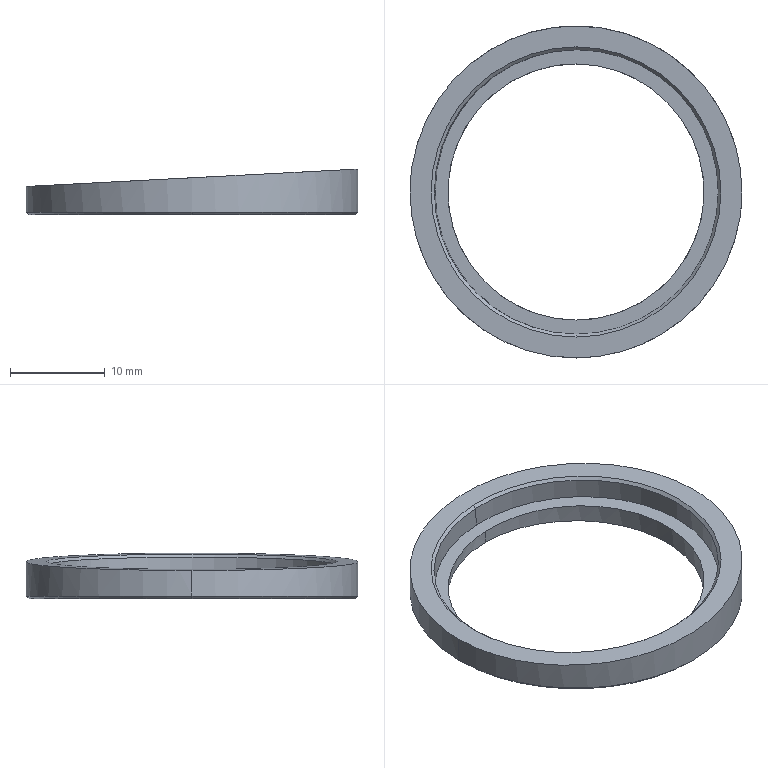Part | STEP file | TCHK-2D-D30-BB-4.stp.STEP | 1 solid | 14 faces | box 35 x 35 x 4.834 mm | volume 1185 mm3 | cylinder 6 | cone 5 | plane 3 | commonest cylinder face diameters 27 x2 30 x2 35 x2
STEP:
#1=CARTESIAN_POINT('',(0.,13.5,0.));
#2=VERTEX_POINT('',#1);
#3=CARTESIAN_POINT('',(0.,-13.5,0.));
#4=VERTEX_POINT('',#3);
#5=CARTESIAN_POINT('',(0.,0.,0.));
#6=DIRECTION('',(0.,0.,-1.));
#7=DIRECTION('',(0.,1.,0.));
#8=AXIS2_PLACEMENT_3D('',#5,#6,#7);
#9=CIRCLE('',#8,13.5);
#10=EDGE_CURVE('',#2,#4,#9,.T.);
#11=ORIENTED_EDGE('',*,*,#10,.F.);
#12=CARTESIAN_POINT('',(0.,0.,0.));
#13=DIRECTION('',(0.,0.,-1.));
#14=DIRECTION('',(0.,-1.,0.));
#15=AXIS2_PLACEMENT_3D('',#12,#13,#14);
#16=CIRCLE('',#15,13.5);
#17=EDGE_CURVE('',#4,#2,#16,.T.);
#18=ORIENTED_EDGE('',*,*,#17,.F.);
#19=EDGE_LOOP('',(#11,#18));
#20=FACE_BOUND('',#19,.T.);
#21=CARTESIAN_POINT('',(17.2,0.,0.000000446));
#22=VERTEX_POINT('',#21);
#23=CARTESIAN_POINT('',(0.,-17.2,0.000000446));
#24=VERTEX_POINT('',#23);
#25=CARTESIAN_POINT('',(0.,0.,0.000000446));
#26=DIRECTION('',(0.,0.,-1.));
#27=DIRECTION('',(1.,0.,0.));
#28=AXIS2_PLACEMENT_3D('',#25,#26,#27);
#29=CIRCLE('',#28,17.2);
#30=EDGE_CURVE('',#22,#24,#29,.T.);
#31=ORIENTED_EDGE('',*,*,#30,.T.);
#32=CARTESIAN_POINT('',(-17.2,0.,0.000000446));
#33=VERTEX_POINT('',#32);
#34=CARTESIAN_POINT('',(0.,0.,0.000000446));
#35=DIRECTION('',(0.,0.,-1.));
#36=DIRECTION('',(1.,0.,0.));
#37=AXIS2_PLACEMENT_3D('',#34,#35,#36);
#38=CIRCLE('',#37,17.2);
#39=EDGE_CURVE('',#24,#33,#38,.T.);
#40=ORIENTED_EDGE('',*,*,#39,.T.);
#41=CARTESIAN_POINT('',(0.,0.,0.000000446));
#42=DIRECTION('',(0.,0.,-1.));
#43=DIRECTION('',(-1.,0.,0.));
#44=AXIS2_PLACEMENT_3D('',#41,#42,#43);
#45=CIRCLE('',#44,17.2);
#46=EDGE_CURVE('',#33,#22,#45,.T.);
#47=ORIENTED_EDGE('',*,*,#46,.T.);
#48=EDGE_LOOP('',(#31,#40,#47));
#49=FACE_OUTER_BOUND('',#48,.T.);
#50=CARTESIAN_POINT('',(0.,0.,0.));
#51=DIRECTION('',(0.,0.,1.));
#52=DIRECTION('',(1.,0.,0.));
#53=AXIS2_PLACEMENT_3D('',#50,#51,#52);
#54=PLANE('',#53);
#55=ADVANCED_FACE('',(#20,#49),#54,.F.);
#56=CARTESIAN_POINT('',(-17.5,0.,0.3));
#57=VERTEX_POINT('',#56);
#58=CARTESIAN_POINT('',(-17.2,-0.000000003,0.000000796));
#59=DIRECTION('',(-0.7071,0.000000001,0.7071));
#60=VECTOR('',#59,1000.);
#61=LINE('',#58,#60);
#62=EDGE_CURVE('',#33,#57,#61,.T.);
#63=ORIENTED_EDGE('',*,*,#62,.T.);
#64=CARTESIAN_POINT('',(17.5,0.,0.3));
#65=VERTEX_POINT('',#64);
#66=CARTESIAN_POINT('',(0.,0.,0.3));
#67=DIRECTION('',(0.,0.,-1.));
#68=DIRECTION('',(-1.,0.,0.));
#69=AXIS2_PLACEMENT_3D('',#66,#67,#68);
#70=CIRCLE('',#69,17.5);
#71=EDGE_CURVE('',#57,#65,#70,.T.);
#72=ORIENTED_EDGE('',*,*,#71,.T.);
#73=CARTESIAN_POINT('',(17.2,0.000000003,0.000000796));
#74=DIRECTION('',(0.7071,-0.000000001,0.7071));
#75=VECTOR('',#74,1000.);
#76=LINE('',#73,#75);
#77=EDGE_CURVE('',#22,#65,#76,.T.);
#78=ORIENTED_EDGE('',*,*,#77,.F.);
#79=ORIENTED_EDGE('',*,*,#46,.F.);
#80=EDGE_LOOP('',(#63,#72,#78,#79));
#81=FACE_OUTER_BOUND('',#80,.T.);
#82=CARTESIAN_POINT('',(0.,0.,0.15));
#83=DIRECTION('',(0.,0.,1.));
#84=DIRECTION('',(0.,-1.,0.));
#85=AXIS2_PLACEMENT_3D('',#82,#83,#84);
#86=CONICAL_SURFACE('',#85,17.35,0.7854);
#87=ADVANCED_FACE('',(#81),#86,.T.);
#88=CARTESIAN_POINT('',(0.,-17.5,0.3));
#89=VERTEX_POINT('',#88);
#90=CARTESIAN_POINT('',(0.,-17.35,0.15));
#91=DIRECTION('',(0.,-0.7071,0.7071));
#92=VECTOR('',#91,1000.);
#93=LINE('',#90,#92);
#94=EDGE_CURVE('',#24,#89,#93,.T.);
#95=ORIENTED_EDGE('',*,*,#94,.F.);
#96=ORIENTED_EDGE('',*,*,#30,.F.);
#97=ORIENTED_EDGE('',*,*,#77,.T.);
#98=CARTESIAN_POINT('',(0.,0.,0.3));
#99=DIRECTION('',(0.,0.,-1.));
#100=DIRECTION('',(1.,0.,0.));
#101=AXIS2_PLACEMENT_3D('',#98,#99,#100);
#102=CIRCLE('',#101,17.5);
#103=EDGE_CURVE('',#65,#89,#102,.T.);
#104=ORIENTED_EDGE('',*,*,#103,.T.);
#105=EDGE_LOOP('',(#95,#96,#97,#104));
#106=FACE_OUTER_BOUND('',#105,.T.);
#107=CARTESIAN_POINT('',(0.,0.,0.15));
#108=DIRECTION('',(0.,0.,1.));
#109=DIRECTION('',(0.,-1.,0.));
#110=AXIS2_PLACEMENT_3D('',#107,#108,#109);
#111=CONICAL_SURFACE('',#110,17.35,0.7854);
#112=ADVANCED_FACE('',(#106),#111,.T.);
#113=CARTESIAN_POINT('',(17.5,0.,4.834));
#114=VERTEX_POINT('',#113);
#115=CARTESIAN_POINT('',(17.5,0.000000002,0.3));
#116=DIRECTION('',(0.000000134,0.,1.));
#117=VECTOR('',#116,1000.);
#118=LINE('',#115,#117);
#119=EDGE_CURVE('',#65,#114,#118,.T.);
#120=ORIENTED_EDGE('',*,*,#119,.T.);
#121=CARTESIAN_POINT('',(-17.5,0.,3.));
#122=VERTEX_POINT('',#121);
#123=CARTESIAN_POINT('',(-17.5,0.,3.));
#124=CARTESIAN_POINT('',(-17.5,-0.5353,3.));
#125=CARTESIAN_POINT('',(-17.463,-1.335,3.002));
#126=CARTESIAN_POINT('',(-17.357,-2.262,3.007));
#127=CARTESIAN_POINT('',(-17.288,-2.723,3.011));
#128=CARTESIAN_POINT('',(-17.249,-2.954,3.013));
#129=CARTESIAN_POINT('',(-17.232,-3.053,3.014));
#130=CARTESIAN_POINT('',(-17.22,-3.119,3.015));
#131=CARTESIAN_POINT('',(-17.214,-3.149,3.015));
#132=CARTESIAN_POINT('',(-17.105,-3.742,3.021));
#133=CARTESIAN_POINT('',(-16.91,-4.568,3.031));
#134=CARTESIAN_POINT('',(-16.614,-5.512,3.046));
#135=CARTESIAN_POINT('',(-16.448,-5.978,3.055));
#136=CARTESIAN_POINT('',(-16.361,-6.21,3.06));
#137=CARTESIAN_POINT('',(-16.323,-6.31,3.062));
#138=CARTESIAN_POINT('',(-16.297,-6.376,3.063));
#139=CARTESIAN_POINT('',(-16.285,-6.407,3.064));
#140=CARTESIAN_POINT('',(-16.054,-6.991,3.076));
#141=CARTESIAN_POINT('',(-15.687,-7.796,3.095));
#142=CARTESIAN_POINT('',(-15.191,-8.698,3.121));
#143=CARTESIAN_POINT('',(-14.925,-9.14,3.135));
#144=CARTESIAN_POINT('',(-14.807,-9.328,3.141));
#145=CARTESIAN_POINT('',(-14.728,-9.452,3.145));
#146=CARTESIAN_POINT('',(-14.689,-9.513,3.147));
#147=CARTESIAN_POINT('',(-13.987,-10.587,3.184));
#148=CARTESIAN_POINT('',(-13.228,-11.521,3.224));
#149=CARTESIAN_POINT('',(-11.948,-12.801,3.291));
#150=CARTESIAN_POINT('',(-11.278,-13.406,3.326));
#151=CARTESIAN_POINT('',(-10.444,-14.047,3.37));
#152=CARTESIAN_POINT('',(-10.015,-14.353,3.392));
#153=CARTESIAN_POINT('',(-9.828,-14.48,3.402));
#154=CARTESIAN_POINT('',(-9.702,-14.564,3.409));
#155=CARTESIAN_POINT('',(-9.638,-14.607,3.412));
#156=CARTESIAN_POINT('',(-9.082,-14.971,3.441));
#157=CARTESIAN_POINT('',(-8.319,-15.416,3.481));
#158=CARTESIAN_POINT('',(-7.393,-15.867,3.53));
#159=CARTESIAN_POINT('',(-6.92,-16.075,3.554));
#160=CARTESIAN_POINT('',(-6.682,-16.174,3.567));
#161=CARTESIAN_POINT('',(-6.579,-16.216,3.572));
#162=CARTESIAN_POINT('',(-6.51,-16.244,3.576));
#163=CARTESIAN_POINT('',(-6.475,-16.258,3.578));
#164=CARTESIAN_POINT('',(-5.915,-16.48,3.607));
#165=CARTESIAN_POINT('',(-5.113,-16.754,3.649));
#166=CARTESIAN_POINT('',(-4.155,-17.004,3.699));
#167=CARTESIAN_POINT('',(-3.672,-17.112,3.725));
#168=CARTESIAN_POINT('',(-3.428,-17.161,3.737));
#169=CARTESIAN_POINT('',(-3.324,-17.181,3.743));
#170=CARTESIAN_POINT('',(-3.254,-17.195,3.747));
#171=CARTESIAN_POINT('',(-3.217,-17.202,3.749));
#172=CARTESIAN_POINT('',(-2.133,-17.403,3.805));
#173=CARTESIAN_POINT('',(-1.07,-17.5,3.861));
#174=CARTESIAN_POINT('',(0.535,-17.5,3.945));
#175=CARTESIAN_POINT('',(1.334,-17.464,3.987));
#176=CARTESIAN_POINT('',(2.261,-17.357,4.036));
#177=CARTESIAN_POINT('',(2.723,-17.288,4.06));
#178=CARTESIAN_POINT('',(2.954,-17.249,4.072));
#179=CARTESIAN_POINT('',(3.053,-17.232,4.077));
#180=CARTESIAN_POINT('',(3.119,-17.22,4.081));
#181=CARTESIAN_POINT('',(3.149,-17.214,4.082));
#182=CARTESIAN_POINT('',(3.743,-17.105,4.113));
#183=CARTESIAN_POINT('',(4.569,-16.91,4.157));
#184=CARTESIAN_POINT('',(5.512,-16.614,4.206));
#185=CARTESIAN_POINT('',(5.978,-16.448,4.23));
#186=CARTESIAN_POINT('',(6.21,-16.361,4.243));
#187=CARTESIAN_POINT('',(6.31,-16.323,4.248));
#188=CARTESIAN_POINT('',(6.376,-16.297,4.251));
#189=CARTESIAN_POINT('',(6.407,-16.285,4.253));
#190=CARTESIAN_POINT('',(6.992,-16.054,4.284));
#191=CARTESIAN_POINT('',(7.796,-15.687,4.326));
#192=CARTESIAN_POINT('',(8.698,-15.19,4.373));
#193=CARTESIAN_POINT('',(9.14,-14.925,4.396));
#194=CARTESIAN_POINT('',(9.328,-14.807,4.406));
#195=CARTESIAN_POINT('',(9.452,-14.728,4.413));
#196=CARTESIAN_POINT('',(9.513,-14.689,4.416));
#197=CARTESIAN_POINT('',(10.587,-13.987,4.472));
#198=CARTESIAN_POINT('',(11.521,-13.228,4.521));
#199=CARTESIAN_POINT('',(12.801,-11.948,4.588));
#200=CARTESIAN_POINT('',(13.405,-11.278,4.62));
#201=CARTESIAN_POINT('',(14.047,-10.444,4.653));
#202=CARTESIAN_POINT('',(14.353,-10.015,4.669));
#203=CARTESIAN_POINT('',(14.48,-9.828,4.676));
#204=CARTESIAN_POINT('',(14.564,-9.702,4.68));
#205=CARTESIAN_POINT('',(14.607,-9.638,4.683));
#206=CARTESIAN_POINT('',(14.971,-9.082,4.702));
#207=CARTESIAN_POINT('',(15.416,-8.319,4.725));
#208=CARTESIAN_POINT('',(15.867,-7.393,4.749));
#209=CARTESIAN_POINT('',(16.075,-6.92,4.76));
#210=CARTESIAN_POINT('',(16.174,-6.682,4.765));
#211=CARTESIAN_POINT('',(16.216,-6.579,4.767));
#212=CARTESIAN_POINT('',(16.244,-6.51,4.768));
#213=CARTESIAN_POINT('',(16.258,-6.475,4.769));
#214=CARTESIAN_POINT('',(16.48,-5.915,4.781));
#215=CARTESIAN_POINT('',(16.754,-5.112,4.795));
#216=CARTESIAN_POINT('',(17.004,-4.155,4.808));
#217=CARTESIAN_POINT('',(17.112,-3.672,4.814));
#218=CARTESIAN_POINT('',(17.161,-3.428,4.817));
#219=CARTESIAN_POINT('',(17.181,-3.324,4.818));
#220=CARTESIAN_POINT('',(17.195,-3.254,4.818));
#221=CARTESIAN_POINT('',(17.202,-3.217,4.819));
#222=CARTESIAN_POINT('',(17.403,-2.133,4.829));
#223=CARTESIAN_POINT('',(17.5,-1.071,4.834));
#224=CARTESIAN_POINT('',(17.5,0.,4.834));
#225=B_SPLINE_CURVE_WITH_KNOTS('',3,(#123,#124,#125,#126,#127,#128,#129,#130,#131,#132,#133,#134,#135,#136,#137,#138,#139,#140,#141,#142,#143,#144,#145,#146,#147,#148,#149,#150,#151,#152,#153,#154,#155,#156,#157,#158,#159,#160,#161,#162,#163,#164,#165,#166,#167,#168,#169,#170,#171,#172,#173,#174,#175,#176,#177,#178,#179,#180,#181,#182,#183,#184,#185,#186,#187,#188,#189,#190,#191,#192,#193,#194,#195,#196,#197,#198,#199,#200,#201,#202,#203,#204,#205,#206,#207,#208,#209,#210,#211,#212,#213,#214,#215,#216,#217,#218,#219,#220,#221,#222,#223,#224),.UNSPECIFIED.,.F.,.F.,(4,1,1,1,1,2,2,1,1,1,1,2,2,1,1,1,2,2,2,1,1,1,2,2,1,1,1,1,2,2,1,1,1,1,2,2,2,1,1,1,1,2,2,1,1,1,1,2,2,1,1,1,2,2,2,1,1,1,2,2,1,1,1,1,2,2,1,1,1,1,2,2,4),(0.,0.03125,0.04687,0.05469,0.05859,0.06055,0.0625,0.09375,0.1094,0.1172,0.1211,0.123,0.125,0.1562,0.1719,0.1797,0.1836,0.1875,0.25,0.2812,0.2969,0.3047,0.3086,0.3125,0.3437,0.3594,0.3672,0.3711,0.373,0.375,0.4062,0.4219,0.4297,0.4336,0.4355,0.4375,0.5,0.5312,0.5469,0.5547,0.5586,0.5605,0.5625,0.5937,0.6094,0.6172,0.6211,0.623,0.625,0.6562,0.6719,0.6797,0.6836,0.6875,0.75,0.7812,0.7969,0.8047,0.8086,0.8125,0.8437,0.8594,0.8672,0.8711,0.873,0.875,0.9062,0.9219,0.9297,0.9336,0.9355,0.9375,1.),.UNSPECIFIED.);
#226=EDGE_CURVE('',#122,#114,#225,.T.);
#227=ORIENTED_EDGE('',*,*,#226,.F.);
#228=CARTESIAN_POINT('',(-17.5,-0.000000002,0.3));
#229=DIRECTION('',(-0.000000225,0.000000001,1.));
#230=VECTOR('',#229,1000.);
#231=LINE('',#228,#230);
#232=EDGE_CURVE('',#57,#122,#231,.T.);
#233=ORIENTED_EDGE('',*,*,#232,.F.);
#234=CARTESIAN_POINT('',(0.,0.,0.3));
#235=DIRECTION('',(0.,0.,-1.));
#236=DIRECTION('',(1.,0.,0.));
#237=AXIS2_PLACEMENT_3D('',#234,#235,#236);
#238=CIRCLE('',#237,17.5);
#239=EDGE_CURVE('',#89,#57,#238,.T.);
#240=ORIENTED_EDGE('',*,*,#239,.F.);
#241=ORIENTED_EDGE('',*,*,#103,.F.);
#242=EDGE_LOOP('',(#120,#227,#233,#240,#241));
#243=FACE_OUTER_BOUND('',#242,.T.);
#244=CARTESIAN_POINT('',(0.,0.,0.));
#245=DIRECTION('',(0.,0.,1.));
#246=DIRECTION('',(1.,0.,0.));
#247=AXIS2_PLACEMENT_3D('',#244,#245,#246);
#248=CYLINDRICAL_SURFACE('',#247,17.5);
#249=ADVANCED_FACE('',(#243),#248,.T.);
#250=ORIENTED_EDGE('',*,*,#232,.T.);
#251=CARTESIAN_POINT('',(17.5,0.,4.834));
#252=CARTESIAN_POINT('',(17.5,0.5353,4.834));
#253=CARTESIAN_POINT('',(17.463,1.335,4.832));
#254=CARTESIAN_POINT('',(17.357,2.262,4.827));
#255=CARTESIAN_POINT('',(17.288,2.723,4.823));
#256=CARTESIAN_POINT('',(17.249,2.954,4.821));
#257=CARTESIAN_POINT('',(17.232,3.053,4.82));
#258=CARTESIAN_POINT('',(17.22,3.119,4.82));
#259=CARTESIAN_POINT('',(17.214,3.149,4.819));
#260=CARTESIAN_POINT('',(17.105,3.742,4.814));
#261=CARTESIAN_POINT('',(16.91,4.568,4.803));
#262=CARTESIAN_POINT('',(16.614,5.512,4.788));
#263=CARTESIAN_POINT('',(16.448,5.978,4.779));
#264=CARTESIAN_POINT('',(16.361,6.21,4.775));
#265=CARTESIAN_POINT('',(16.323,6.31,4.773));
#266=CARTESIAN_POINT('',(16.297,6.376,4.771));
#267=CARTESIAN_POINT('',(16.285,6.407,4.771));
#268=CARTESIAN_POINT('',(16.054,6.991,4.758));
#269=CARTESIAN_POINT('',(15.687,7.796,4.739));
#270=CARTESIAN_POINT('',(15.191,8.698,4.713));
#271=CARTESIAN_POINT('',(14.925,9.14,4.699));
#272=CARTESIAN_POINT('',(14.807,9.328,4.693));
#273=CARTESIAN_POINT('',(14.728,9.452,4.689));
#274=CARTESIAN_POINT('',(14.689,9.513,4.687));
#275=CARTESIAN_POINT('',(13.987,10.587,4.65));
#276=CARTESIAN_POINT('',(13.228,11.521,4.61));
#277=CARTESIAN_POINT('',(11.948,12.801,4.543));
#278=CARTESIAN_POINT('',(11.278,13.406,4.508));
#279=CARTESIAN_POINT('',(10.444,14.047,4.464));
#280=CARTESIAN_POINT('',(10.015,14.353,4.442));
#281=CARTESIAN_POINT('',(9.828,14.48,4.432));
#282=CARTESIAN_POINT('',(9.702,14.564,4.426));
#283=CARTESIAN_POINT('',(9.638,14.607,4.422));
#284=CARTESIAN_POINT('',(9.082,14.971,4.393));
#285=CARTESIAN_POINT('',(8.319,15.416,4.353));
#286=CARTESIAN_POINT('',(7.393,15.867,4.305));
#287=CARTESIAN_POINT('',(6.92,16.075,4.28));
#288=CARTESIAN_POINT('',(6.682,16.174,4.267));
#289=CARTESIAN_POINT('',(6.579,16.216,4.262));
#290=CARTESIAN_POINT('',(6.51,16.244,4.258));
#291=CARTESIAN_POINT('',(6.475,16.258,4.256));
#292=CARTESIAN_POINT('',(5.915,16.48,4.227));
#293=CARTESIAN_POINT('',(5.113,16.754,4.185));
#294=CARTESIAN_POINT('',(4.155,17.004,4.135));
#295=CARTESIAN_POINT('',(3.672,17.112,4.11));
#296=CARTESIAN_POINT('',(3.428,17.161,4.097));
#297=CARTESIAN_POINT('',(3.324,17.181,4.091));
#298=CARTESIAN_POINT('',(3.254,17.195,4.088));
#299=CARTESIAN_POINT('',(3.217,17.202,4.086));
#300=CARTESIAN_POINT('',(2.133,17.403,4.029));
#301=CARTESIAN_POINT('',(1.07,17.5,3.973));
#302=CARTESIAN_POINT('',(-0.535,17.5,3.889));
#303=CARTESIAN_POINT('',(-1.334,17.464,3.847));
#304=CARTESIAN_POINT('',(-2.261,17.357,3.799));
#305=CARTESIAN_POINT('',(-2.723,17.288,3.774));
#306=CARTESIAN_POINT('',(-2.954,17.249,3.762));
#307=CARTESIAN_POINT('',(-3.053,17.232,3.757));
#308=CARTESIAN_POINT('',(-3.119,17.22,3.754));
#309=CARTESIAN_POINT('',(-3.149,17.214,3.752));
#310=CARTESIAN_POINT('',(-3.743,17.105,3.721));
#311=CARTESIAN_POINT('',(-4.569,16.91,3.678));
#312=CARTESIAN_POINT('',(-5.512,16.614,3.628));
#313=CARTESIAN_POINT('',(-5.978,16.448,3.604));
#314=CARTESIAN_POINT('',(-6.21,16.361,3.592));
#315=CARTESIAN_POINT('',(-6.31,16.323,3.586));
#316=CARTESIAN_POINT('',(-6.376,16.297,3.583));
#317=CARTESIAN_POINT('',(-6.407,16.285,3.581));
#318=CARTESIAN_POINT('',(-6.992,16.054,3.551));
#319=CARTESIAN_POINT('',(-7.796,15.687,3.509));
#320=CARTESIAN_POINT('',(-8.698,15.19,3.461));
#321=CARTESIAN_POINT('',(-9.14,14.925,3.438));
#322=CARTESIAN_POINT('',(-9.328,14.807,3.428));
#323=CARTESIAN_POINT('',(-9.452,14.728,3.422));
#324=CARTESIAN_POINT('',(-9.513,14.689,3.419));
#325=CARTESIAN_POINT('',(-10.587,13.987,3.362));
#326=CARTESIAN_POINT('',(-11.521,13.228,3.313));
#327=CARTESIAN_POINT('',(-12.801,11.948,3.246));
#328=CARTESIAN_POINT('',(-13.405,11.278,3.215));
#329=CARTESIAN_POINT('',(-14.047,10.444,3.181));
#330=CARTESIAN_POINT('',(-14.353,10.015,3.165));
#331=CARTESIAN_POINT('',(-14.48,9.828,3.158));
#332=CARTESIAN_POINT('',(-14.564,9.702,3.154));
#333=CARTESIAN_POINT('',(-14.607,9.638,3.152));
#334=CARTESIAN_POINT('',(-14.971,9.082,3.133));
#335=CARTESIAN_POINT('',(-15.416,8.319,3.109));
#336=CARTESIAN_POINT('',(-15.867,7.393,3.086));
#337=CARTESIAN_POINT('',(-16.075,6.92,3.075));
#338=CARTESIAN_POINT('',(-16.174,6.682,3.069));
#339=CARTESIAN_POINT('',(-16.216,6.579,3.067));
#340=CARTESIAN_POINT('',(-16.244,6.51,3.066));
#341=CARTESIAN_POINT('',(-16.258,6.475,3.065));
#342=CARTESIAN_POINT('',(-16.48,5.915,3.053));
#343=CARTESIAN_POINT('',(-16.754,5.112,3.039));
#344=CARTESIAN_POINT('',(-17.004,4.155,3.026));
#345=CARTESIAN_POINT('',(-17.112,3.672,3.02));
#346=CARTESIAN_POINT('',(-17.161,3.428,3.018));
#347=CARTESIAN_POINT('',(-17.181,3.324,3.017));
#348=CARTESIAN_POINT('',(-17.195,3.254,3.016));
#349=CARTESIAN_POINT('',(-17.202,3.217,3.016));
#350=CARTESIAN_POINT('',(-17.403,2.133,3.005));
#351=CARTESIAN_POINT('',(-17.5,1.071,3.));
#352=CARTESIAN_POINT('',(-17.5,0.,3.));
#353=B_SPLINE_CURVE_WITH_KNOTS('',3,(#251,#252,#253,#254,#255,#256,#257,#258,#259,#260,#261,#262,#263,#264,#265,#266,#267,#268,#269,#270,#271,#272,#273,#274,#275,#276,#277,#278,#279,#280,#281,#282,#283,#284,#285,#286,#287,#288,#289,#290,#291,#292,#293,#294,#295,#296,#297,#298,#299,#300,#301,#302,#303,#304,#305,#306,#307,#308,#309,#310,#311,#312,#313,#314,#315,#316,#317,#318,#319,#320,#321,#322,#323,#324,#325,#326,#327,#328,#329,#330,#331,#332,#333,#334,#335,#336,#337,#338,#339,#340,#341,#342,#343,#344,#345,#346,#347,#348,#349,#350,#351,#352),.UNSPECIFIED.,.F.,.F.,(4,1,1,1,1,2,2,1,1,1,1,2,2,1,1,1,2,2,2,1,1,1,2,2,1,1,1,1,2,2,1,1,1,1,2,2,2,1,1,1,1,2,2,1,1,1,1,2,2,1,1,1,2,2,2,1,1,1,2,2,1,1,1,1,2,2,1,1,1,1,2,2,4),(0.,0.03125,0.04688,0.05469,0.05859,0.06055,0.0625,0.09375,0.1094,0.1172,0.1211,0.123,0.125,0.1563,0.1719,0.1797,0.1836,0.1875,0.25,0.2813,0.2969,0.3047,0.3086,0.3125,0.3438,0.3594,0.3672,0.3711,0.373,0.375,0.4063,0.4219,0.4297,0.4336,0.4355,0.4375,0.5,0.5313,0.5469,0.5547,0.5586,0.5605,0.5625,0.5938,0.6094,0.6172,0.6211,0.623,0.625,0.6563,0.6719,0.6797,0.6836,0.6875,0.75,0.7813,0.7969,0.8047,0.8086,0.8125,0.8438,0.8594,0.8672,0.8711,0.873,0.875,0.9063,0.9219,0.9297,0.9336,0.9355,0.9375,1.),.UNSPECIFIED.);
#354=EDGE_CURVE('',#114,#122,#353,.T.);
#355=ORIENTED_EDGE('',*,*,#354,.F.);
#356=ORIENTED_EDGE('',*,*,#119,.F.);
#357=ORIENTED_EDGE('',*,*,#71,.F.);
#358=EDGE_LOOP('',(#250,#355,#356,#357));
#359=FACE_OUTER_BOUND('',#358,.T.);
#360=CARTESIAN_POINT('',(0.,0.,0.));
#361=DIRECTION('',(0.,0.,1.));
#362=DIRECTION('',(1.,0.,0.));
#363=AXIS2_PLACEMENT_3D('',#360,#361,#362);
#364=CYLINDRICAL_SURFACE('',#363,17.5);
#365=ADVANCED_FACE('',(#359),#364,.T.);
#366=CARTESIAN_POINT('',(0.000000029,-15.3,3.917));
#367=VERTEX_POINT('',#366);
#368=CARTESIAN_POINT('',(0.000000029,15.3,3.917));
#369=VERTEX_POINT('',#368);
#370=CARTESIAN_POINT('',(0.000000029,0.,3.917));
#371=DIRECTION('',(0.05234,0.,-0.9986));
#372=DIRECTION('',(0.,-1.,0.));
#373=AXIS2_PLACEMENT_3D('',#370,#371,#372);
#374=CIRCLE('',#373,15.3);
#375=EDGE_CURVE('',#367,#369,#374,.T.);
#376=ORIENTED_EDGE('',*,*,#375,.T.);
#377=CARTESIAN_POINT('',(0.000000029,0.,3.917));
#378=DIRECTION('',(0.05234,0.,-0.9986));
#379=DIRECTION('',(0.,1.,0.));
#380=AXIS2_PLACEMENT_3D('',#377,#378,#379);
#381=CIRCLE('',#380,15.3);
#382=EDGE_CURVE('',#369,#367,#381,.T.);
#383=ORIENTED_EDGE('',*,*,#382,.T.);
#384=EDGE_LOOP('',(#376,#383));
#385=FACE_BOUND('',#384,.T.);
#386=ORIENTED_EDGE('',*,*,#226,.T.);
#387=ORIENTED_EDGE('',*,*,#354,.T.);
#388=EDGE_LOOP('',(#386,#387));
#389=FACE_OUTER_BOUND('',#388,.T.);
#390=CARTESIAN_POINT('',(17.5,-50.,4.834));
#391=DIRECTION('',(0.05234,0.,-0.9986));
#392=DIRECTION('',(0.,-1.,0.));
#393=AXIS2_PLACEMENT_3D('',#390,#391,#392);
#394=PLANE('',#393);
#395=ADVANCED_FACE('',(#385,#389),#394,.F.);
#396=CARTESIAN_POINT('',(0.0157,15.,3.618));
#397=VERTEX_POINT('',#396);
#398=CARTESIAN_POINT('',(-0.000000016,15.3,3.917));
#399=DIRECTION('',(0.03701,-0.7071,-0.7061));
#400=VECTOR('',#399,1000.);
#401=LINE('',#398,#400);
#402=EDGE_CURVE('',#369,#397,#401,.T.);
#403=ORIENTED_EDGE('',*,*,#402,.T.);
#404=CARTESIAN_POINT('',(0.0157,-15.,3.618));
#405=VERTEX_POINT('',#404);
#406=CARTESIAN_POINT('',(0.0157,0.,3.618));
#407=DIRECTION('',(0.05234,0.,-0.9986));
#408=DIRECTION('',(0.,1.,0.));
#409=AXIS2_PLACEMENT_3D('',#406,#407,#408);
#410=CIRCLE('',#409,15.);
#411=EDGE_CURVE('',#397,#405,#410,.T.);
#412=ORIENTED_EDGE('',*,*,#411,.T.);
#413=CARTESIAN_POINT('',(-0.000000009,-15.3,3.917));
#414=DIRECTION('',(0.03701,0.7071,-0.7061));
#415=VECTOR('',#414,1000.);
#416=LINE('',#413,#415);
#417=EDGE_CURVE('',#367,#405,#416,.T.);
#418=ORIENTED_EDGE('',*,*,#417,.F.);
#419=ORIENTED_EDGE('',*,*,#382,.F.);
#420=EDGE_LOOP('',(#403,#412,#418,#419));
#421=FACE_OUTER_BOUND('',#420,.T.);
#422=CARTESIAN_POINT('',(0.00785,0.,3.767));
#423=DIRECTION('',(-0.05234,0.,0.9986));
#424=DIRECTION('',(0.,-1.,0.));
#425=AXIS2_PLACEMENT_3D('',#422,#423,#424);
#426=CONICAL_SURFACE('',#425,15.15,0.7854);
#427=ADVANCED_FACE('',(#421),#426,.F.);
#428=ORIENTED_EDGE('',*,*,#417,.T.);
#429=CARTESIAN_POINT('',(0.0157,0.,3.618));
#430=DIRECTION('',(0.05234,0.,-0.9986));
#431=DIRECTION('',(0.,-1.,0.));
#432=AXIS2_PLACEMENT_3D('',#429,#430,#431);
#433=CIRCLE('',#432,15.);
#434=EDGE_CURVE('',#405,#397,#433,.T.);
#435=ORIENTED_EDGE('',*,*,#434,.T.);
#436=ORIENTED_EDGE('',*,*,#402,.F.);
#437=ORIENTED_EDGE('',*,*,#375,.F.);
#438=EDGE_LOOP('',(#428,#435,#436,#437));
#439=FACE_OUTER_BOUND('',#438,.T.);
#440=CARTESIAN_POINT('',(0.00785,0.,3.767));
#441=DIRECTION('',(-0.05234,0.,0.9986));
#442=DIRECTION('',(0.,-1.,0.));
#443=AXIS2_PLACEMENT_3D('',#440,#441,#442);
#444=CONICAL_SURFACE('',#443,15.15,0.7854);
#445=ADVANCED_FACE('',(#439),#444,.F.);
#446=CARTESIAN_POINT('',(0.1308,-15.,1.421));
#447=VERTEX_POINT('',#446);
#448=CARTESIAN_POINT('',(0.0157,-15.,3.618));
#449=DIRECTION('',(0.05234,-0.00000008,-0.9986));
#450=VECTOR('',#449,1000.);
#451=LINE('',#448,#450);
#452=EDGE_CURVE('',#405,#447,#451,.T.);
#453=ORIENTED_EDGE('',*,*,#452,.T.);
#454=CARTESIAN_POINT('',(0.1308,15.,1.421));
#455=VERTEX_POINT('',#454);
#456=CARTESIAN_POINT('',(0.1308,0.,1.421));
#457=DIRECTION('',(0.05234,0.,-0.9986));
#458=DIRECTION('',(0.,-1.,0.));
#459=AXIS2_PLACEMENT_3D('',#456,#457,#458);
#460=CIRCLE('',#459,15.);
#461=EDGE_CURVE('',#447,#455,#460,.T.);
#462=ORIENTED_EDGE('',*,*,#461,.T.);
#463=CARTESIAN_POINT('',(0.0157,15.,3.618));
#464=DIRECTION('',(0.05234,0.00000008,-0.9986));
#465=VECTOR('',#464,1000.);
#466=LINE('',#463,#465);
#467=EDGE_CURVE('',#397,#455,#466,.T.);
#468=ORIENTED_EDGE('',*,*,#467,.F.);
#469=ORIENTED_EDGE('',*,*,#434,.F.);
#470=EDGE_LOOP('',(#453,#462,#468,#469));
#471=FACE_OUTER_BOUND('',#470,.T.);
#472=CARTESIAN_POINT('',(0.,0.,3.917));
#473=DIRECTION('',(-0.05234,0.,0.9986));
#474=DIRECTION('',(0.,1.,0.));
#475=AXIS2_PLACEMENT_3D('',#472,#473,#474);
#476=CYLINDRICAL_SURFACE('',#475,15.);
#477=ADVANCED_FACE('',(#471),#476,.F.);
#478=ORIENTED_EDGE('',*,*,#467,.T.);
#479=CARTESIAN_POINT('',(0.1308,0.,1.421));
#480=DIRECTION('',(0.05234,0.,-0.9986));
#481=DIRECTION('',(0.,1.,0.));
#482=AXIS2_PLACEMENT_3D('',#479,#480,#481);
#483=CIRCLE('',#482,15.);
#484=EDGE_CURVE('',#455,#447,#483,.T.);
#485=ORIENTED_EDGE('',*,*,#484,.T.);
#486=ORIENTED_EDGE('',*,*,#452,.F.);
#487=ORIENTED_EDGE('',*,*,#411,.F.);
#488=EDGE_LOOP('',(#478,#485,#486,#487));
#489=FACE_OUTER_BOUND('',#488,.T.);
#490=CARTESIAN_POINT('',(0.,0.,3.917));
#491=DIRECTION('',(-0.05234,0.,0.9986));
#492=DIRECTION('',(0.,1.,0.));
#493=AXIS2_PLACEMENT_3D('',#490,#491,#492);
#494=CYLINDRICAL_SURFACE('',#493,15.);
#495=ADVANCED_FACE('',(#489),#494,.F.);
#496=CARTESIAN_POINT('',(0.,13.5,1.414));
#497=VERTEX_POINT('',#496);
#498=CARTESIAN_POINT('',(0.,-13.5,1.414));
#499=VERTEX_POINT('',#498);
#500=CARTESIAN_POINT('',(0.,13.5,1.414));
#501=CARTESIAN_POINT('',(0.4129,13.5,1.435));
#502=CARTESIAN_POINT('',(1.03,13.472,1.468));
#503=CARTESIAN_POINT('',(1.745,13.39,1.505));
#504=CARTESIAN_POINT('',(2.101,13.336,1.524));
#505=CARTESIAN_POINT('',(2.279,13.306,1.533));
#506=CARTESIAN_POINT('',(2.355,13.293,1.537));
#507=CARTESIAN_POINT('',(2.406,13.284,1.54));
#508=CARTESIAN_POINT('',(2.43,13.28,1.541));
#509=CARTESIAN_POINT('',(2.887,13.195,1.565));
#510=CARTESIAN_POINT('',(3.524,13.045,1.598));
#511=CARTESIAN_POINT('',(4.252,12.816,1.637));
#512=CARTESIAN_POINT('',(4.612,12.689,1.655));
#513=CARTESIAN_POINT('',(4.791,12.622,1.665));
#514=CARTESIAN_POINT('',(4.867,12.592,1.669));
#515=CARTESIAN_POINT('',(4.918,12.572,1.671));
#516=CARTESIAN_POINT('',(4.943,12.563,1.673));
#517=CARTESIAN_POINT('',(5.393,12.384,1.696));
#518=CARTESIAN_POINT('',(6.014,12.102,1.729));
#519=CARTESIAN_POINT('',(6.71,11.719,1.765));
#520=CARTESIAN_POINT('',(7.051,11.513,1.783));
#521=CARTESIAN_POINT('',(7.196,11.423,1.791));
#522=CARTESIAN_POINT('',(7.292,11.362,1.796));
#523=CARTESIAN_POINT('',(7.339,11.331,1.798));
#524=CARTESIAN_POINT('',(8.167,10.79,1.842));
#525=CARTESIAN_POINT('',(8.887,10.204,1.879));
#526=CARTESIAN_POINT('',(9.875,9.217,1.931));
#527=CARTESIAN_POINT('',(10.341,8.7,1.956));
#528=CARTESIAN_POINT('',(10.837,8.057,1.982));
#529=CARTESIAN_POINT('',(11.072,7.726,1.994));
#530=CARTESIAN_POINT('',(11.17,7.581,1.999));
#531=CARTESIAN_POINT('',(11.235,7.485,2.003));
#532=CARTESIAN_POINT('',(11.268,7.435,2.004));
#533=CARTESIAN_POINT('',(11.549,7.006,2.019));
#534=CARTESIAN_POINT('',(11.892,6.418,2.037));
#535=CARTESIAN_POINT('',(12.24,5.703,2.055));
#536=CARTESIAN_POINT('',(12.4,5.339,2.064));
#537=CARTESIAN_POINT('',(12.477,5.155,2.068));
#538=CARTESIAN_POINT('',(12.51,5.075,2.069));
#539=CARTESIAN_POINT('',(12.531,5.022,2.07));
#540=CARTESIAN_POINT('',(12.542,4.995,2.071));
#541=CARTESIAN_POINT('',(12.713,4.563,2.08));
#542=CARTESIAN_POINT('',(12.924,3.944,2.091));
#543=CARTESIAN_POINT('',(13.117,3.205,2.101));
#544=CARTESIAN_POINT('',(13.2,2.832,2.106));
#545=CARTESIAN_POINT('',(13.239,2.645,2.108));
#546=CARTESIAN_POINT('',(13.254,2.564,2.108));
#547=CARTESIAN_POINT('',(13.265,2.51,2.109));
#548=CARTESIAN_POINT('',(13.27,2.482,2.109));
#549=CARTESIAN_POINT('',(13.425,1.645,2.117));
#550=CARTESIAN_POINT('',(13.5,0.8248,2.121));
#551=CARTESIAN_POINT('',(13.5,-0.4124,2.121));
#552=CARTESIAN_POINT('',(13.472,-1.029,2.12));
#553=CARTESIAN_POINT('',(13.39,-1.744,2.115));
#554=CARTESIAN_POINT('',(13.336,-2.101,2.113));
#555=CARTESIAN_POINT('',(13.306,-2.279,2.111));
#556=CARTESIAN_POINT('',(13.293,-2.355,2.11));
#557=CARTESIAN_POINT('',(13.284,-2.406,2.11));
#558=CARTESIAN_POINT('',(13.28,-2.43,2.11));
#559=CARTESIAN_POINT('',(13.195,-2.887,2.105));
#560=CARTESIAN_POINT('',(13.045,-3.524,2.097));
#561=CARTESIAN_POINT('',(12.816,-4.252,2.085));
#562=CARTESIAN_POINT('',(12.689,-4.612,2.079));
#563=CARTESIAN_POINT('',(12.622,-4.791,2.075));
#564=CARTESIAN_POINT('',(12.592,-4.867,2.074));
#565=CARTESIAN_POINT('',(12.572,-4.918,2.073));
#566=CARTESIAN_POINT('',(12.563,-4.943,2.072));
#567=CARTESIAN_POINT('',(12.384,-5.393,2.063));
#568=CARTESIAN_POINT('',(12.102,-6.014,2.048));
#569=CARTESIAN_POINT('',(11.718,-6.71,2.028));
#570=CARTESIAN_POINT('',(11.513,-7.051,2.017));
#571=CARTESIAN_POINT('',(11.423,-7.196,2.012));
#572=CARTESIAN_POINT('',(11.362,-7.292,2.009));
#573=CARTESIAN_POINT('',(11.331,-7.339,2.008));
#574=CARTESIAN_POINT('',(10.79,-8.167,1.979));
#575=CARTESIAN_POINT('',(10.204,-8.887,1.948));
#576=CARTESIAN_POINT('',(9.217,-9.875,1.897));
#577=CARTESIAN_POINT('',(8.7,-10.341,1.87));
#578=CARTESIAN_POINT('',(8.057,-10.837,1.836));
#579=CARTESIAN_POINT('',(7.726,-11.072,1.819));
#580=CARTESIAN_POINT('',(7.581,-11.17,1.811));
#581=CARTESIAN_POINT('',(7.485,-11.235,1.806));
#582=CARTESIAN_POINT('',(7.435,-11.268,1.803));
#583=CARTESIAN_POINT('',(7.006,-11.549,1.781));
#584=CARTESIAN_POINT('',(6.418,-11.892,1.75));
#585=CARTESIAN_POINT('',(5.703,-12.24,1.713));
#586=CARTESIAN_POINT('',(5.338,-12.401,1.693));
#587=CARTESIAN_POINT('',(5.154,-12.477,1.684));
#588=CARTESIAN_POINT('',(5.075,-12.51,1.68));
#589=CARTESIAN_POINT('',(5.022,-12.531,1.677));
#590=CARTESIAN_POINT('',(4.995,-12.542,1.675));
#591=CARTESIAN_POINT('',(4.563,-12.713,1.653));
#592=CARTESIAN_POINT('',(3.944,-12.924,1.62));
#593=CARTESIAN_POINT('',(3.206,-13.117,1.582));
#594=CARTESIAN_POINT('',(2.832,-13.2,1.562));
#595=CARTESIAN_POINT('',(2.645,-13.239,1.552));
#596=CARTESIAN_POINT('',(2.564,-13.254,1.548));
#597=CARTESIAN_POINT('',(2.51,-13.265,1.545));
#598=CARTESIAN_POINT('',(2.482,-13.27,1.544));
#599=CARTESIAN_POINT('',(1.645,-13.425,1.5));
#600=CARTESIAN_POINT('',(0.8265,-13.5,1.457));
#601=CARTESIAN_POINT('',(0.,-13.5,1.414));
#602=B_SPLINE_CURVE_WITH_KNOTS('',3,(#500,#501,#502,#503,#504,#505,#506,#507,#508,#509,#510,#511,#512,#513,#514,#515,#516,#517,#518,#519,#520,#521,#522,#523,#524,#525,#526,#527,#528,#529,#530,#531,#532,#533,#534,#535,#536,#537,#538,#539,#540,#541,#542,#543,#544,#545,#546,#547,#548,#549,#550,#551,#552,#553,#554,#555,#556,#557,#558,#559,#560,#561,#562,#563,#564,#565,#566,#567,#568,#569,#570,#571,#572,#573,#574,#575,#576,#577,#578,#579,#580,#581,#582,#583,#584,#585,#586,#587,#588,#589,#590,#591,#592,#593,#594,#595,#596,#597,#598,#599,#600,#601),.UNSPECIFIED.,.F.,.F.,(4,1,1,1,1,2,2,1,1,1,1,2,2,1,1,1,2,2,2,1,1,1,2,2,1,1,1,1,2,2,1,1,1,1,2,2,2,1,1,1,1,2,2,1,1,1,1,2,2,1,1,1,2,2,2,1,1,1,2,2,1,1,1,1,2,2,1,1,1,1,2,2,4),(0.,0.03125,0.04688,0.05469,0.05859,0.06055,0.0625,0.09375,0.1094,0.1172,0.1211,0.123,0.125,0.1563,0.1719,0.1797,0.1836,0.1875,0.25,0.2813,0.2969,0.3047,0.3086,0.3125,0.3438,0.3594,0.3672,0.3711,0.373,0.375,0.4063,0.4219,0.4297,0.4336,0.4355,0.4375,0.5,0.5313,0.5469,0.5547,0.5586,0.5605,0.5625,0.5938,0.6094,0.6172,0.6211,0.623,0.625,0.6563,0.6719,0.6797,0.6836,0.6875,0.75,0.7812,0.7969,0.8047,0.8086,0.8125,0.8437,0.8594,0.8672,0.8711,0.873,0.875,0.9063,0.9219,0.9297,0.9336,0.9355,0.9375,1.),.UNSPECIFIED.);
#603=EDGE_CURVE('',#497,#499,#602,.T.);
#604=ORIENTED_EDGE('',*,*,#603,.T.);
#605=CARTESIAN_POINT('',(0.,-13.5,1.414));
#606=CARTESIAN_POINT('',(-0.4129,-13.5,1.392));
#607=CARTESIAN_POINT('',(-1.03,-13.472,1.36));
#608=CARTESIAN_POINT('',(-1.745,-13.39,1.322));
#609=CARTESIAN_POINT('',(-2.101,-13.336,1.304));
#610=CARTESIAN_POINT('',(-2.279,-13.306,1.294));
#611=CARTESIAN_POINT('',(-2.355,-13.293,1.29));
#612=CARTESIAN_POINT('',(-2.406,-13.284,1.288));
#613=CARTESIAN_POINT('',(-2.43,-13.28,1.286));
#614=CARTESIAN_POINT('',(-2.887,-13.195,1.262));
#615=CARTESIAN_POINT('',(-3.524,-13.045,1.229));
#616=CARTESIAN_POINT('',(-4.252,-12.816,1.191));
#617=CARTESIAN_POINT('',(-4.612,-12.689,1.172));
#618=CARTESIAN_POINT('',(-4.791,-12.622,1.163));
#619=CARTESIAN_POINT('',(-4.867,-12.592,1.159));
#620=CARTESIAN_POINT('',(-4.918,-12.572,1.156));
#621=CARTESIAN_POINT('',(-4.943,-12.563,1.155));
#622=CARTESIAN_POINT('',(-5.393,-12.384,1.131));
#623=CARTESIAN_POINT('',(-6.014,-12.102,1.099));
#624=CARTESIAN_POINT('',(-6.71,-11.719,1.062));
#625=CARTESIAN_POINT('',(-7.051,-11.513,1.044));
#626=CARTESIAN_POINT('',(-7.196,-11.423,1.037));
#627=CARTESIAN_POINT('',(-7.292,-11.362,1.032));
#628=CARTESIAN_POINT('',(-7.339,-11.331,1.029));
#629=CARTESIAN_POINT('',(-8.167,-10.79,0.9857));
#630=CARTESIAN_POINT('',(-8.887,-10.204,0.9479));
#631=CARTESIAN_POINT('',(-9.875,-9.217,0.8962));
#632=CARTESIAN_POINT('',(-10.341,-8.7,0.8717));
#633=CARTESIAN_POINT('',(-10.837,-8.057,0.8458));
#634=CARTESIAN_POINT('',(-11.072,-7.726,0.8334));
#635=CARTESIAN_POINT('',(-11.17,-7.581,0.8283));
#636=CARTESIAN_POINT('',(-11.235,-7.485,0.8249));
#637=CARTESIAN_POINT('',(-11.268,-7.435,0.8232));
#638=CARTESIAN_POINT('',(-11.549,-7.006,0.8085));
#639=CARTESIAN_POINT('',(-11.892,-6.418,0.7905));
#640=CARTESIAN_POINT('',(-12.24,-5.703,0.7722));
#641=CARTESIAN_POINT('',(-12.4,-5.339,0.7638));
#642=CARTESIAN_POINT('',(-12.477,-5.155,0.7598));
#643=CARTESIAN_POINT('',(-12.51,-5.075,0.7581));
#644=CARTESIAN_POINT('',(-12.531,-5.022,0.757));
#645=CARTESIAN_POINT('',(-12.542,-4.995,0.7564));
#646=CARTESIAN_POINT('',(-12.713,-4.563,0.7474));
#647=CARTESIAN_POINT('',(-12.924,-3.944,0.7364));
#648=CARTESIAN_POINT('',(-13.117,-3.205,0.7263));
#649=CARTESIAN_POINT('',(-13.2,-2.832,0.7219));
#650=CARTESIAN_POINT('',(-13.239,-2.645,0.7199));
#651=CARTESIAN_POINT('',(-13.254,-2.564,0.7191));
#652=CARTESIAN_POINT('',(-13.265,-2.51,0.7185));
#653=CARTESIAN_POINT('',(-13.27,-2.482,0.7183));
#654=CARTESIAN_POINT('',(-13.425,-1.645,0.7101));
#655=CARTESIAN_POINT('',(-13.5,-0.8248,0.7062));
#656=CARTESIAN_POINT('',(-13.5,0.4124,0.7062));
#657=CARTESIAN_POINT('',(-13.472,1.029,0.7077));
#658=CARTESIAN_POINT('',(-13.39,1.744,0.712));
#659=CARTESIAN_POINT('',(-13.336,2.101,0.7148));
#660=CARTESIAN_POINT('',(-13.306,2.279,0.7163));
#661=CARTESIAN_POINT('',(-13.293,2.355,0.717));
#662=CARTESIAN_POINT('',(-13.284,2.406,0.7175));
#663=CARTESIAN_POINT('',(-13.28,2.43,0.7178));
#664=CARTESIAN_POINT('',(-13.195,2.887,0.7222));
#665=CARTESIAN_POINT('',(-13.045,3.524,0.73));
#666=CARTESIAN_POINT('',(-12.816,4.252,0.742));
#667=CARTESIAN_POINT('',(-12.689,4.612,0.7487));
#668=CARTESIAN_POINT('',(-12.622,4.791,0.7522));
#669=CARTESIAN_POINT('',(-12.592,4.867,0.7538));
#670=CARTESIAN_POINT('',(-12.572,4.918,0.7548));
#671=CARTESIAN_POINT('',(-12.563,4.943,0.7553));
#672=CARTESIAN_POINT('',(-12.384,5.393,0.7647));
#673=CARTESIAN_POINT('',(-12.102,6.014,0.7795));
#674=CARTESIAN_POINT('',(-11.718,6.71,0.7996));
#675=CARTESIAN_POINT('',(-11.513,7.051,0.8103));
#676=CARTESIAN_POINT('',(-11.423,7.196,0.8151));
#677=CARTESIAN_POINT('',(-11.362,7.292,0.8183));
#678=CARTESIAN_POINT('',(-11.331,7.339,0.8199));
#679=CARTESIAN_POINT('',(-10.79,8.167,0.8482));
#680=CARTESIAN_POINT('',(-10.204,8.887,0.8789));
#681=CARTESIAN_POINT('',(-9.217,9.875,0.9307));
#682=CARTESIAN_POINT('',(-8.7,10.341,0.9578));
#683=CARTESIAN_POINT('',(-8.057,10.837,0.9915));
#684=CARTESIAN_POINT('',(-7.726,11.072,1.009));
#685=CARTESIAN_POINT('',(-7.581,11.17,1.016));
#686=CARTESIAN_POINT('',(-7.485,11.235,1.021));
#687=CARTESIAN_POINT('',(-7.435,11.268,1.024));
#688=CARTESIAN_POINT('',(-7.006,11.549,1.047));
#689=CARTESIAN_POINT('',(-6.418,11.892,1.077));
#690=CARTESIAN_POINT('',(-5.703,12.24,1.115));
#691=CARTESIAN_POINT('',(-5.338,12.401,1.134));
#692=CARTESIAN_POINT('',(-5.154,12.477,1.144));
#693=CARTESIAN_POINT('',(-5.075,12.51,1.148));
#694=CARTESIAN_POINT('',(-5.022,12.531,1.15));
#695=CARTESIAN_POINT('',(-4.995,12.542,1.152));
#696=CARTESIAN_POINT('',(-4.563,12.713,1.175));
#697=CARTESIAN_POINT('',(-3.944,12.924,1.207));
#698=CARTESIAN_POINT('',(-3.206,13.117,1.246));
#699=CARTESIAN_POINT('',(-2.832,13.2,1.265));
#700=CARTESIAN_POINT('',(-2.645,13.239,1.275));
#701=CARTESIAN_POINT('',(-2.564,13.254,1.279));
#702=CARTESIAN_POINT('',(-2.51,13.265,1.282));
#703=CARTESIAN_POINT('',(-2.482,13.27,1.284));
#704=CARTESIAN_POINT('',(-1.645,13.425,1.327));
#705=CARTESIAN_POINT('',(-0.8265,13.5,1.37));
#706=CARTESIAN_POINT('',(0.,13.5,1.414));
#707=B_SPLINE_CURVE_WITH_KNOTS('',3,(#605,#606,#607,#608,#609,#610,#611,#612,#613,#614,#615,#616,#617,#618,#619,#620,#621,#622,#623,#624,#625,#626,#627,#628,#629,#630,#631,#632,#633,#634,#635,#636,#637,#638,#639,#640,#641,#642,#643,#644,#645,#646,#647,#648,#649,#650,#651,#652,#653,#654,#655,#656,#657,#658,#659,#660,#661,#662,#663,#664,#665,#666,#667,#668,#669,#670,#671,#672,#673,#674,#675,#676,#677,#678,#679,#680,#681,#682,#683,#684,#685,#686,#687,#688,#689,#690,#691,#692,#693,#694,#695,#696,#697,#698,#699,#700,#701,#702,#703,#704,#705,#706),.UNSPECIFIED.,.F.,.F.,(4,1,1,1,1,2,2,1,1,1,1,2,2,1,1,1,2,2,2,1,1,1,2,2,1,1,1,1,2,2,1,1,1,1,2,2,2,1,1,1,1,2,2,1,1,1,1,2,2,1,1,1,2,2,2,1,1,1,2,2,1,1,1,1,2,2,1,1,1,1,2,2,4),(0.,0.03125,0.04688,0.05469,0.05859,0.06055,0.0625,0.09375,0.1094,0.1172,0.1211,0.123,0.125,0.1563,0.1719,0.1797,0.1836,0.1875,0.25,0.2813,0.2969,0.3047,0.3086,0.3125,0.3438,0.3594,0.3672,0.3711,0.373,0.375,0.4063,0.4219,0.4297,0.4336,0.4355,0.4375,0.5,0.5313,0.5469,0.5547,0.5586,0.5605,0.5625,0.5938,0.6094,0.6172,0.6211,0.623,0.625,0.6563,0.6719,0.6797,0.6836,0.6875,0.75,0.7813,0.7969,0.8047,0.8086,0.8125,0.8438,0.8594,0.8672,0.8711,0.873,0.875,0.9063,0.9219,0.9297,0.9336,0.9355,0.9375,1.),.UNSPECIFIED.);
#708=EDGE_CURVE('',#499,#497,#707,.T.);
#709=ORIENTED_EDGE('',*,*,#708,.T.);
#710=EDGE_LOOP('',(#604,#709));
#711=FACE_BOUND('',#710,.T.);
#712=ORIENTED_EDGE('',*,*,#484,.F.);
#713=ORIENTED_EDGE('',*,*,#461,.F.);
#714=EDGE_LOOP('',(#712,#713));
#715=FACE_OUTER_BOUND('',#714,.T.);
#716=CARTESIAN_POINT('',(-0.07389,-50.,1.41));
#717=DIRECTION('',(-0.05234,0.,0.9986));
#718=DIRECTION('',(0.,1.,0.));
#719=AXIS2_PLACEMENT_3D('',#716,#717,#718);
#720=PLANE('',#719);
#721=ADVANCED_FACE('',(#711,#715),#720,.T.);
#722=CARTESIAN_POINT('',(0.,13.5,0.));
#723=DIRECTION('',(0.,0.,1.));
#724=VECTOR('',#723,1000.);
#725=LINE('',#722,#724);
#726=EDGE_CURVE('',#2,#497,#725,.T.);
#727=ORIENTED_EDGE('',*,*,#726,.T.);
#728=ORIENTED_EDGE('',*,*,#708,.F.);
#729=CARTESIAN_POINT('',(0.,-13.5,0.));
#730=DIRECTION('',(0.,0.,1.));
#731=VECTOR('',#730,1000.);
#732=LINE('',#729,#731);
#733=EDGE_CURVE('',#4,#499,#732,.T.);
#734=ORIENTED_EDGE('',*,*,#733,.F.);
#735=ORIENTED_EDGE('',*,*,#17,.T.);
#736=EDGE_LOOP('',(#727,#728,#734,#735));
#737=FACE_OUTER_BOUND('',#736,.T.);
#738=CARTESIAN_POINT('',(0.,0.,0.));
#739=DIRECTION('',(0.,0.,-1.));
#740=DIRECTION('',(0.,-1.,0.));
#741=AXIS2_PLACEMENT_3D('',#738,#739,#740);
#742=CYLINDRICAL_SURFACE('',#741,13.5);
#743=ADVANCED_FACE('',(#737),#742,.F.);
#744=ORIENTED_EDGE('',*,*,#733,.T.);
#745=ORIENTED_EDGE('',*,*,#603,.F.);
#746=ORIENTED_EDGE('',*,*,#726,.F.);
#747=ORIENTED_EDGE('',*,*,#10,.T.);
#748=EDGE_LOOP('',(#744,#745,#746,#747));
#749=FACE_OUTER_BOUND('',#748,.T.);
#750=CARTESIAN_POINT('',(0.,0.,0.));
#751=DIRECTION('',(0.,0.,-1.));
#752=DIRECTION('',(0.,-1.,0.));
#753=AXIS2_PLACEMENT_3D('',#750,#751,#752);
#754=CYLINDRICAL_SURFACE('',#753,13.5);
#755=ADVANCED_FACE('',(#749),#754,.F.);
#756=ORIENTED_EDGE('',*,*,#39,.F.);
#757=ORIENTED_EDGE('',*,*,#94,.T.);
#758=ORIENTED_EDGE('',*,*,#239,.T.);
#759=ORIENTED_EDGE('',*,*,#62,.F.);
#760=EDGE_LOOP('',(#756,#757,#758,#759));
#761=FACE_OUTER_BOUND('',#760,.T.);
#762=CARTESIAN_POINT('',(0.,0.,0.15));
#763=DIRECTION('',(0.,0.,1.));
#764=DIRECTION('',(0.,-1.,0.));
#765=AXIS2_PLACEMENT_3D('',#762,#763,#764);
#766=CONICAL_SURFACE('',#765,17.35,0.7854);
#767=ADVANCED_FACE('',(#761),#766,.T.);
#768=CLOSED_SHELL('',(#55,#87,#112,#249,#365,#395,#427,#445,#477,#495,#721,#743,#755,#767));
#769=MANIFOLD_SOLID_BREP('',#768);
#770=CARTESIAN_POINT('',(0.,0.,0.));
#771=DIRECTION('',(0.,0.,1.));
#772=DIRECTION('',(1.,0.,0.));
#773=AXIS2_PLACEMENT_3D('',#770,#771,#772);
#774=(LENGTH_UNIT()NAMED_UNIT(*)SI_UNIT(.MILLI.,.METRE.));
#775=UNCERTAINTY_MEASURE_WITH_UNIT(LENGTH_MEASURE(0.00001),#774,'','');
#776=(NAMED_UNIT(*)PLANE_ANGLE_UNIT()SI_UNIT($,.RADIAN.));
#777=(NAMED_UNIT(*)SI_UNIT($,.STERADIAN.)SOLID_ANGLE_UNIT());
#778=(GEOMETRIC_REPRESENTATION_CONTEXT(3)GLOBAL_UNCERTAINTY_ASSIGNED_CONTEXT((#775))GLOBAL_UNIT_ASSIGNED_CONTEXT((#774,#776,#777))REPRESENTATION_CONTEXT('',''));
#779=ADVANCED_BREP_SHAPE_REPRESENTATION('',(#769,#773),#778);